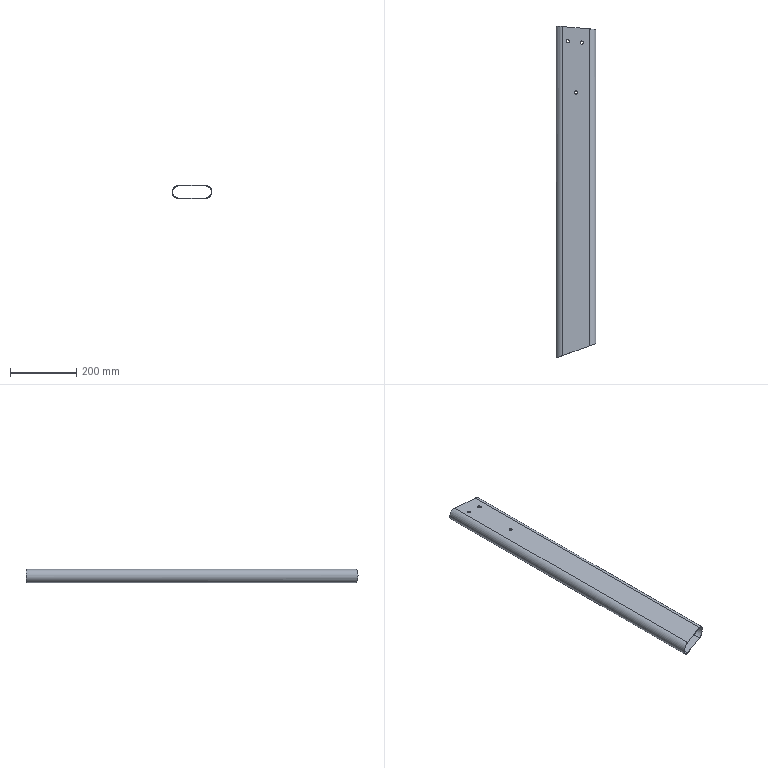Part | STEP file | Q7C0201 | 1 solid | 16 faces | box 120 x 1000 x 40 mm | volume 489501 mm3 | cylinder 10 | plane 6 | commonest cylinder face diameters 10 x6 36.4 x2 40 x2